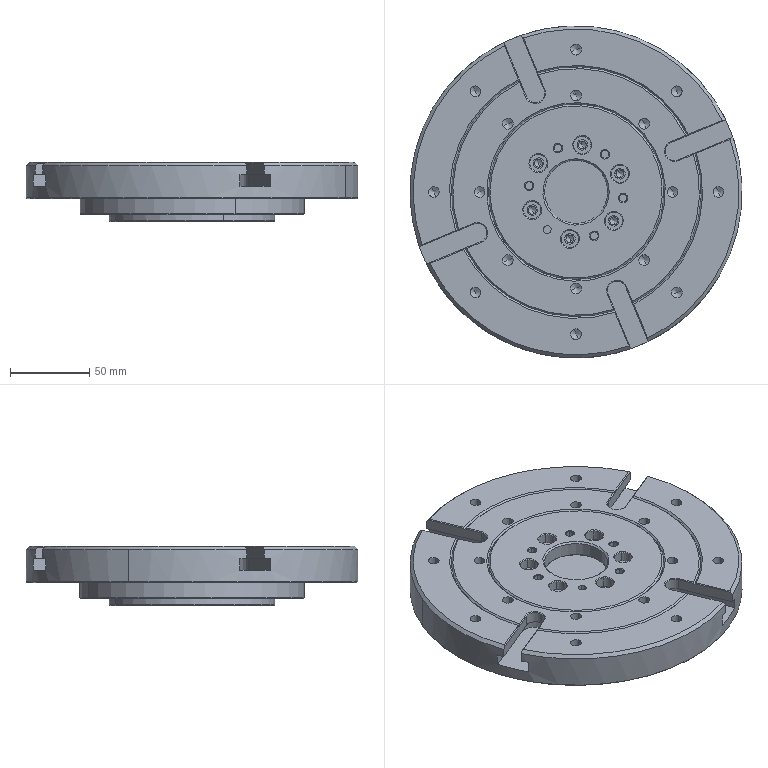NC program | Mastercam | posted with a generic post
Whole program:
%
:0001()
(MATERIAL - ALUMINUM MM - 2024)
(T2|8 CHM |H2)
(T3|2.5 DR |H3)
(T16|M3 X 0.5 RH |H16)
(T18|3.8 DR |H18)
(T6|3 FEMR |H6|D6|WEAR COMP|TOOL DIA. - 3.|XY STOCK TO LEAVE - .05|Z STOCK TO LEAVE - 0.)
(T7|3 FEMF |H7|D7|WEAR COMP|TOOL DIA. - 3.|XY STOCK TO LEAVE - .02|Z STOCK TO LEAVE - 0.)
(T8|26 60DGEA |H8|D8|WEAR COMP|TOOL DIA. - 26.)
N100 G21
N102 G0 G17 G40 G80 G90 G94 G98
N104 G0 G28 G91 Z0.
N106 G0 G28 X0. Y0.
(8 CHM |TOOL - 2|DIA. OFF. - 2|LEN. - 2|TOOL DIA. - 8.)
N108 T2 M6
N110 G0 G54 G90 X-3.35 Y3.35 C0. B0. S2000 M3
N112 G43 H2 Z30.
N114 G81 G98 Z-1.8 R1. F100.
N116 X3.35
N118 X-3.35 Y-3.35
N120 X3.35
N122 G80
N124 X0. Y0.
N126 G81 G98 Z-2.3 R1. F100.
N128 G80
N130 M5
N132 G0 G28 G91 Z0.
N134 G28
N136 M01
N138 G0 G17 G40 G80 G90 G94 G98
N140 G0 G28 G91 Z0.
(2.5 DR |TOOL - 3|DIA. OFF. - 3|LEN. - 3|TOOL DIA. - 2.5)
N142 T3 M6
N144 G0 G54 G90 X-3.35 Y3.35 C0. B0. S2000 M3
N146 G43 H3 Z30.
N148 G83 G98 Z-12. R1. Q2. F100.
N150 X3.35
N152 X-3.35 Y-3.35
N154 X3.35
N156 G80
N158 M5
N160 G0 G28 G91 Z0.
N162 G28
N164 M01
N166 G0 G17 G40 G80 G90 G94 G98
N168 G0 G28 G91 Z0.
(M3 X 0.5 RH |TOOL - 16|DIA. OFF. - 16|LEN. - 16|TOOL DIA. - 3.)
N170 T16 M6
N172 G0 G54 G90 X-3.35 Y3.35 C0. B0. S200 M3
N174 G43 H16 Z30.
N176 G84 G98 Z-5. R1. F100.
N178 X3.35
N180 X-3.35 Y-3.35
N182 X3.35
N184 G80
N186 M5
N188 G0 G28 G91 Z0.
N190 G28
N192 M01
N194 G0 G17 G40 G80 G90 G94 G98
N196 G0 G28 G91 Z0.
(3.8 DR |TOOL - 18|DIA. OFF. - 18|LEN. - 18|TOOL DIA. - 3.8)
N198 T18 M6
N200 G0 G54 G90 X0. Y0. C0. B0. S2000 M3
N202 G43 H18 Z30.
N204 G83 G98 Z-9.142 R1. Q2. F100.
N206 G80
N208 M5
N210 G0 G28 G91 Z0.
N212 G28
N214 M01
N216 G0 G17 G40 G80 G90 G94 G98
N218 G0 G28 G91 Z0.
(3 FEMR |TOOL - 6|DIA. OFF. - 6|LEN. - 6|TOOL DIA. - 3.)
N220 T6 M6
N222 G0 G54 G90 X0. Y0. C0. B0. S3500 M3
N224 G43 H6 Z30.
N226 Z2.
N228 G1 Z-8. F2000.
N230 G41 D6 X.329 F300.
N232 G3 X.34 Y.06 I-.165 J.06
N234 X.329 Y.12 I-.176
N236 X0. Y.35 I-.329 J-.12
N238 X-.35 Y0. J-.35
N240 X0. Y-.35 I.35
N242 X.35 Y0. J.35
N244 X.329 Y.12 I-.35
N246 X.285 Y.203 I-.329 J-.12
N248 X.186 Y.271 I-.143 J-.101
N250 G1 G40 X0. Y0.
N252 G41 D6 X.423
N254 G3 X.437 Y.077 I-.212 J.077
N256 X.423 Y.154 I-.226
N258 X0. Y.45 I-.423 J-.154
N260 X-.45 Y0. J-.45
N262 X0. Y-.45 I.45
N264 X.45 Y0. J.45
N266 X.423 Y.154 I-.45
N268 X.37 Y.256 I-.423 J-.154
N270 X.244 Y.345 I-.185 J-.128
N272 G1 G40 X0. Y0.
N274 G0 Z30.
N276 M5
N278 G0 G28 G91 Z0.
N280 G28
N282 M01
N284 G0 G17 G40 G80 G90 G94 G98
N286 G0 G28 G91 Z0.
(3 FEMF |TOOL - 7|DIA. OFF. - 7|LEN. - 7|TOOL DIA. - 3.)
N288 T7 M6
N290 G0 G54 G90 X0. Y0. C0. B0. S3500 M3
N292 G43 H7 Z30.
N294 Z2.
N296 G1 Z-6.35 F2000.
N298 G41 D7 X.451 F200.
N300 G3 X.465 Y.082 I-.225 J.082
N302 X.451 Y.164 I-.239
N304 X0. Y.48 I-.451 J-.164
N306 X-.48 Y0. J-.48
N308 X0. Y-.48 I.48
N310 X.48 Y0. J.48
N312 X.451 Y.164 I-.48
N314 X.396 Y.272 I-.451 J-.164
N316 X.262 Y.367 I-.198 J-.136
N318 G1 G40 X0. Y0.
N320 G41 D7 X.451
N322 G3 X.465 Y.082 I-.225 J.082
N324 X.451 Y.164 I-.239
N326 X0. Y.48 I-.451 J-.164
N328 X-.48 Y0. J-.48
N330 X0. Y-.48 I.48
N332 X.48 Y0. J.48
N334 X.451 Y.164 I-.48
N336 X.396 Y.272 I-.451 J-.164
N338 X.262 Y.367 I-.198 J-.136
N340 G1 G40 X0. Y0.
N342 G0 Z30.
N344 M5
N346 G0 G28 G91 Z0.
N348 G28
N350 M01
N352 G0 G17 G40 G80 G90 G94 G98
N354 G0 G28 G91 Z0.
(26 60DGEA |TOOL - 8|DIA. OFF. - 8|LEN. - 8|TOOL DIA. - 26.)
M00
N356 T8 M6
N358 G0 G54 G90 X15.4 Y2.884 C180. B-90. S4000 M3
N360 G43 H8 Z50.
N362 Z8.5
N364 G1 Z2.3 F2000.
N366 G41 D8 X12.4 F1000.
N368 G3 X12.3 Y2.784 J-.1
N370 G1 Y-2.784
N372 G3 X12.4 Y-2.884 I.1
N374 G1 G40 X15.4
N376 G0 Z17.5
N378 Y5.094
N380 Z7.25
N382 G1 Z1.05 F2000.
N384 G41 D8 X12.4 F1000.
N386 G3 X12.3 Y4.994 J-.1
N388 G1 Y-4.994
N390 G3 X12.4 Y-5.094 I.1
N392 G1 G40 X15.4
N394 G0 Z16.25
N396 Y6.345
N398 Z6.
N400 G1 Z-.2 F2000.
N402 G41 D8 X12.4 F1000.
N404 G3 X12.3 Y6.245 J-.1
N406 G1 Y-6.245
N408 G3 X12.4 Y-6.345 I.1
N410 G1 G40 X15.4
N412 G0 Z15.
N414 Y7.167
N416 Z4.75
N418 G1 Z-1.45 F2000.
N420 G41 D8 X12.4 F1000.
N422 G3 X12.3 Y7.067 J-.1
N424 G1 Y-7.067
N426 G3 X12.4 Y-7.167 I.1
N428 G1 G40 X15.4
N430 G0 Z13.75
N432 Y7.699
N434 Z3.5
N436 G1 Z-2.7 F2000.
N438 G41 D8 X12.4 F1000.
N440 G3 X12.3 Y7.599 J-.1
N442 G1 Y-7.599
N444 G3 X12.4 Y-7.699 I.1
N446 G1 G40 X15.4
N448 G0 Z12.5
N450 Y8.002
N452 Z2.25
N454 G1 Z-3.95 F2000.
N456 G41 D8 X12.4 F1000.
N458 G3 X12.3 Y7.902 J-.1
N460 G1 Y-7.902
N462 G3 X12.4 Y-8.002 I.1
N464 G1 G40 X15.4
N466 G0 Z11.25
N468 Y8.1
N470 Z1.
N472 G1 Z-5.2 F2000.
N474 G41 D8 X12.4 F1000.
N476 G3 X12.3 Y8. J-.1
N478 G1 Y-8.
N480 G3 X12.4 Y-8.1 I.1
N482 G1 G40 X15.4
N484 G0 Z10.
N486 Y8.002
N488 Z-.25
N490 G1 Z-6.45 F2000.
N492 G41 D8 X12.4 F1000.
N494 G3 X12.3 Y7.902 J-.1
N496 G1 Y-7.902
N498 G3 X12.4 Y-8.002 I.1
N500 G1 G40 X15.4
N502 G0 Z8.75
N504 Y7.699
N506 Z-1.5
N508 G1 Z-7.7 F2000.
N510 G41 D8 X12.4 F1000.
N512 G3 X12.3 Y7.599 J-.1
N514 G1 Y-7.599
N516 G3 X12.4 Y-7.699 I.1
N518 G1 G40 X15.4
N520 G0 Z7.5
N522 Y7.167
N524 Z-2.75
N526 G1 Z-8.95 F2000.
N528 G41 D8 X12.4 F1000.
N530 G3 X12.3 Y7.067 J-.1
N532 G1 Y-7.067
N534 G3 X12.4 Y-7.167 I.1
N536 G1 G40 X15.4
N538 G0 Z6.25
N540 Y6.345
N542 Z-4.
N544 G1 Z-10.2 F2000.
N546 G41 D8 X12.4 F1000.
N548 G3 X12.3 Y6.245 J-.1
N550 G1 Y-6.245
N552 G3 X12.4 Y-6.345 I.1
N554 G1 G40 X15.4
N556 G0 Z5.
N558 Y5.094
N560 Z-5.25
N562 G1 Z-11.45 F2000.
N564 G41 D8 X12.4 F1000.
N566 G3 X12.3 Y4.994 J-.1
N568 G1 Y-4.994
N570 G3 X12.4 Y-5.094 I.1
N572 G1 G40 X15.4
N574 G0 Z3.75
N576 Y2.884
N578 Z-6.5
N580 G1 Z-12.7 F2000.
N582 G41 D8 X12.4 F1000.
N584 G3 X12.3 Y2.784 J-.1
N586 G1 Y-2.784
N588 G3 X12.4 Y-2.884 I.1
N590 G1 G40 X15.4
N592 G0 Z50.
N594 M5
N596 G0 G28 G91 Z0.
N598 G0 G28 X0. Y0.
N600 G28 C0. B0.
G91 G28 Z0. Y0.
N602 M30
%